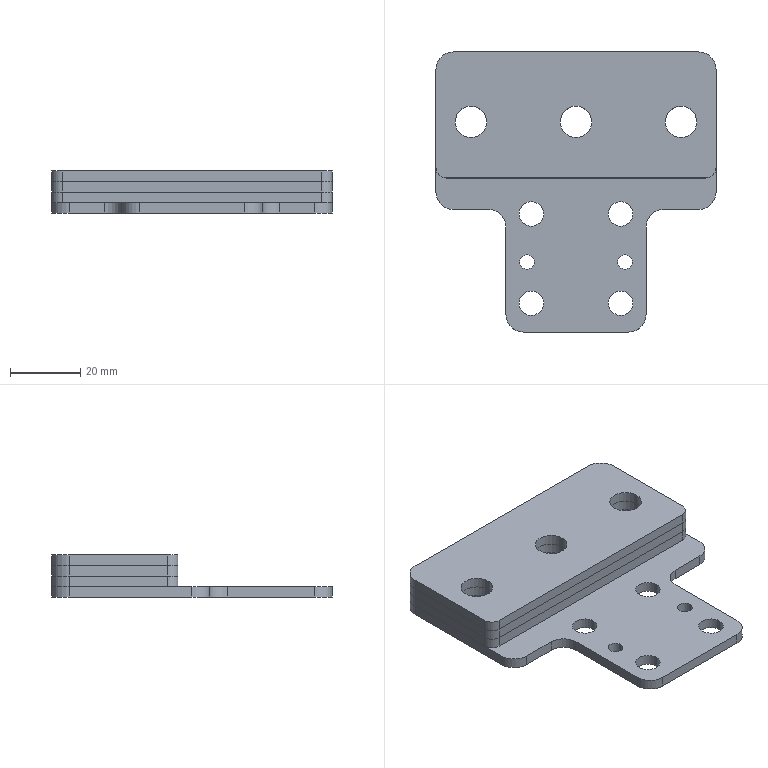Part | SolidWorks | features ICE 5, Fillet 3, Extrusion 1, LPattern 1 | 4 solids | 84 faces | box 80 x 80 x 12 mm | volume 37889 mm3 | cylinder 56 | plane 28 | commonest cylinder face diameters 9 x24 10 x14 7 x8 6 x6 4.2 x4